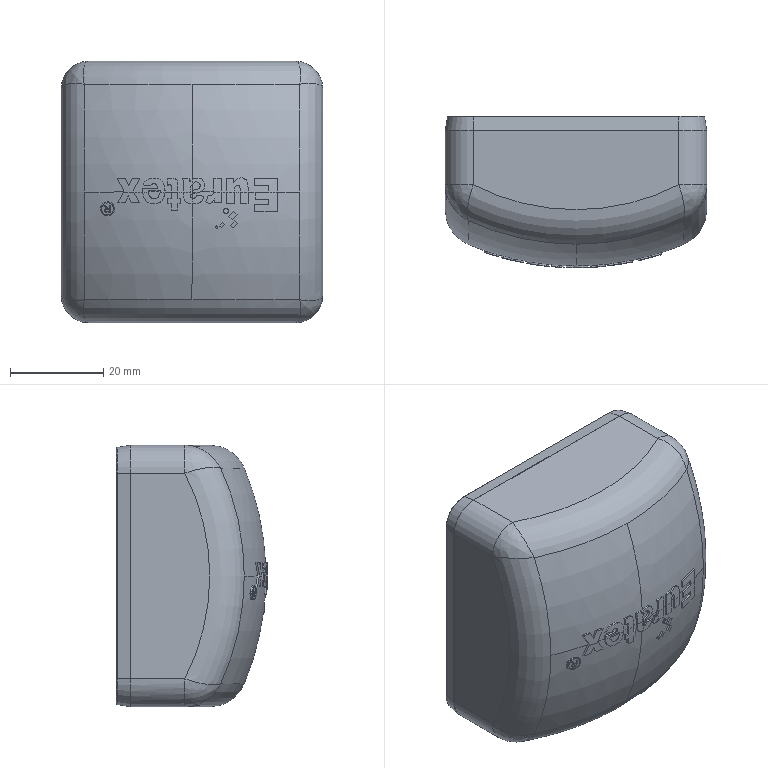Part | STEP file | 101000007581 | 4 solids | 400 faces | box 56 x 32.4 x 56 mm | volume 27988 mm3 | plane 144 | cylinder 93 | torus 62 | sphere 61 | spline 36 | cone 4 | commonest cylinder face diameters 0.4 x43 1 x16 88.667 x8 2.583 x4 6 x4 12 x4